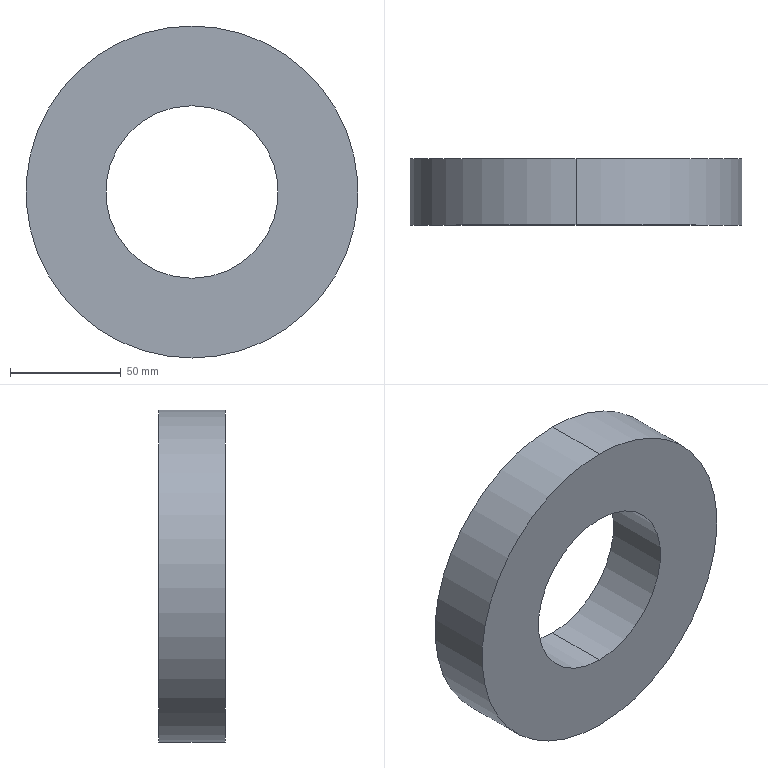Part | STEP file | Take-up roll | 1 solid | 6 faces | box 150 x 30 x 150 mm | volume 386793 mm3 | cylinder 4 | plane 2 | commonest cylinder face diameters 78 x2 150 x2
STEP:
#1=CARTESIAN_POINT('',(0.,0.,0.));
#2=DIRECTION('',(0.,0.,1.));
#3=DIRECTION('',(1.,0.,0.));
#4=AXIS2_PLACEMENT_3D('',#1,#2,#3);
#5=CARTESIAN_POINT('',(0.,15.,-39.));
#6=VERTEX_POINT('',#5);
#7=CARTESIAN_POINT('',(0.,-15.,-39.));
#8=VERTEX_POINT('',#7);
#9=CARTESIAN_POINT('',(0.,15.,-39.));
#10=DIRECTION('',(0.,-1.,0.));
#11=VECTOR('',#10,1.);
#12=LINE('',#9,#11);
#13=CARTESIAN_POINT('',(0.,15.,0.));
#14=DIRECTION('',(0.,-1.,0.));
#15=DIRECTION('',(0.,0.,-1.));
#16=AXIS2_PLACEMENT_3D('',#13,#14,#15);
#17=CYLINDRICAL_SURFACE('',#16,39.);
#18=CARTESIAN_POINT('',(6.283,0.));
#19=DIRECTION('',(0.,1.));
#20=VECTOR('',#19,1.);
#21=LINE('',#18,#20);
#22=(GEOMETRIC_REPRESENTATION_CONTEXT(2)PARAMETRIC_REPRESENTATION_CONTEXT()REPRESENTATION_CONTEXT('',''));
#23=DEFINITIONAL_REPRESENTATION('',(#21),#22);
#24=PCURVE('',#17,#23);
#25=CARTESIAN_POINT('',(0.,15.,0.));
#26=DIRECTION('',(0.,-1.,0.));
#27=DIRECTION('',(0.,0.,-1.));
#28=AXIS2_PLACEMENT_3D('',#25,#26,#27);
#29=CYLINDRICAL_SURFACE('',#28,39.);
#30=CARTESIAN_POINT('',(0.,0.));
#31=DIRECTION('',(0.,1.));
#32=VECTOR('',#31,1.);
#33=LINE('',#30,#32);
#34=(GEOMETRIC_REPRESENTATION_CONTEXT(2)PARAMETRIC_REPRESENTATION_CONTEXT()REPRESENTATION_CONTEXT('',''));
#35=DEFINITIONAL_REPRESENTATION('',(#33),#34);
#36=PCURVE('',#29,#35);
#37=SURFACE_CURVE('',#12,(#24,#36),.PCURVE_S1.);
#38=EDGE_CURVE('',#6,#8,#37,.T.);
#39=ORIENTED_EDGE('',*,*,#38,.T.);
#40=CARTESIAN_POINT('',(0.,-15.,39.));
#41=VERTEX_POINT('',#40);
#42=CARTESIAN_POINT('',(0.,-15.,0.));
#43=DIRECTION('',(0.,-1.,0.));
#44=DIRECTION('',(0.,0.,-1.));
#45=AXIS2_PLACEMENT_3D('',#42,#43,#44);
#46=CIRCLE('',#45,39.);
#47=CARTESIAN_POINT('',(0.,30.));
#48=DIRECTION('',(1.,0.));
#49=VECTOR('',#48,1.);
#50=LINE('',#47,#49);
#51=(GEOMETRIC_REPRESENTATION_CONTEXT(2)PARAMETRIC_REPRESENTATION_CONTEXT()REPRESENTATION_CONTEXT('',''));
#52=DEFINITIONAL_REPRESENTATION('',(#50),#51);
#53=PCURVE('',#17,#52);
#54=CARTESIAN_POINT('',(0.,-15.,0.));
#55=DIRECTION('',(0.,1.,0.));
#56=DIRECTION('',(0.,0.,1.));
#57=AXIS2_PLACEMENT_3D('',#54,#55,#56);
#58=PLANE('',#57);
#59=CARTESIAN_POINT('',(-39.,0.));
#60=CARTESIAN_POINT('',(-39.,67.55));
#61=CARTESIAN_POINT('',(19.5,33.775));
#62=CARTESIAN_POINT('',(78.,0.));
#63=CARTESIAN_POINT('',(19.5,-33.775));
#64=CARTESIAN_POINT('',(-39.,-67.55));
#65=CARTESIAN_POINT('',(-39.,0.));
#66=(BOUNDED_CURVE()B_SPLINE_CURVE(2,(#59,#60,#61,#62,#63,#64,#65),.UNSPECIFIED.,.T.,.F.)B_SPLINE_CURVE_WITH_KNOTS((1,2,2,2,2,1),(-2.094,0.,2.094,4.189,6.283,8.378),.UNSPECIFIED.)CURVE()GEOMETRIC_REPRESENTATION_ITEM()RATIONAL_B_SPLINE_CURVE((1.,0.5,1.,0.5,1.,0.5,1.))REPRESENTATION_ITEM(''));
#67=(GEOMETRIC_REPRESENTATION_CONTEXT(2)PARAMETRIC_REPRESENTATION_CONTEXT()REPRESENTATION_CONTEXT('',''));
#68=DEFINITIONAL_REPRESENTATION('',(#66),#67);
#69=PCURVE('',#58,#68);
#70=SURFACE_CURVE('',#46,(#53,#69),.PCURVE_S1.);
#71=EDGE_CURVE('',#41,#8,#70,.T.);
#72=ORIENTED_EDGE('',*,*,#71,.F.);
#73=CARTESIAN_POINT('',(0.,15.,39.));
#74=VERTEX_POINT('',#73);
#75=CARTESIAN_POINT('',(0.,15.,39.));
#76=DIRECTION('',(0.,-1.,0.));
#77=VECTOR('',#76,1.);
#78=LINE('',#75,#77);
#79=CARTESIAN_POINT('',(3.142,0.));
#80=DIRECTION('',(0.,1.));
#81=VECTOR('',#80,1.);
#82=LINE('',#79,#81);
#83=(GEOMETRIC_REPRESENTATION_CONTEXT(2)PARAMETRIC_REPRESENTATION_CONTEXT()REPRESENTATION_CONTEXT('',''));
#84=DEFINITIONAL_REPRESENTATION('',(#82),#83);
#85=PCURVE('',#17,#84);
#86=CARTESIAN_POINT('',(3.142,0.));
#87=DIRECTION('',(0.,1.));
#88=VECTOR('',#87,1.);
#89=LINE('',#86,#88);
#90=(GEOMETRIC_REPRESENTATION_CONTEXT(2)PARAMETRIC_REPRESENTATION_CONTEXT()REPRESENTATION_CONTEXT('',''));
#91=DEFINITIONAL_REPRESENTATION('',(#89),#90);
#92=PCURVE('',#29,#91);
#93=SURFACE_CURVE('',#78,(#85,#92),.PCURVE_S1.);
#94=EDGE_CURVE('',#74,#41,#93,.T.);
#95=ORIENTED_EDGE('',*,*,#94,.F.);
#96=CARTESIAN_POINT('',(0.,15.,0.));
#97=DIRECTION('',(0.,-1.,0.));
#98=DIRECTION('',(0.,0.,-1.));
#99=AXIS2_PLACEMENT_3D('',#96,#97,#98);
#100=CIRCLE('',#99,39.);
#101=CARTESIAN_POINT('',(0.,0.));
#102=DIRECTION('',(1.,0.));
#103=VECTOR('',#102,1.);
#104=LINE('',#101,#103);
#105=(GEOMETRIC_REPRESENTATION_CONTEXT(2)PARAMETRIC_REPRESENTATION_CONTEXT()REPRESENTATION_CONTEXT('',''));
#106=DEFINITIONAL_REPRESENTATION('',(#104),#105);
#107=PCURVE('',#17,#106);
#108=CARTESIAN_POINT('',(0.,15.,0.));
#109=DIRECTION('',(0.,1.,0.));
#110=DIRECTION('',(0.,0.,1.));
#111=AXIS2_PLACEMENT_3D('',#108,#109,#110);
#112=PLANE('',#111);
#113=CARTESIAN_POINT('',(-39.,0.));
#114=CARTESIAN_POINT('',(-39.,67.55));
#115=CARTESIAN_POINT('',(19.5,33.775));
#116=CARTESIAN_POINT('',(78.,0.));
#117=CARTESIAN_POINT('',(19.5,-33.775));
#118=CARTESIAN_POINT('',(-39.,-67.55));
#119=CARTESIAN_POINT('',(-39.,0.));
#120=(BOUNDED_CURVE()B_SPLINE_CURVE(2,(#113,#114,#115,#116,#117,#118,#119),.UNSPECIFIED.,.T.,.F.)B_SPLINE_CURVE_WITH_KNOTS((1,2,2,2,2,1),(-2.094,0.,2.094,4.189,6.283,8.378),.UNSPECIFIED.)CURVE()GEOMETRIC_REPRESENTATION_ITEM()RATIONAL_B_SPLINE_CURVE((1.,0.5,1.,0.5,1.,0.5,1.))REPRESENTATION_ITEM(''));
#121=(GEOMETRIC_REPRESENTATION_CONTEXT(2)PARAMETRIC_REPRESENTATION_CONTEXT()REPRESENTATION_CONTEXT('',''));
#122=DEFINITIONAL_REPRESENTATION('',(#120),#121);
#123=PCURVE('',#112,#122);
#124=SURFACE_CURVE('',#100,(#107,#123),.PCURVE_S1.);
#125=EDGE_CURVE('',#74,#6,#124,.T.);
#126=ORIENTED_EDGE('',*,*,#125,.T.);
#127=EDGE_LOOP('',(#39,#72,#95,#126));
#128=FACE_BOUND('',#127,.F.);
#129=ADVANCED_FACE('',(#128),#17,.F.);
#130=CARTESIAN_POINT('',(0.,15.,75.));
#131=VERTEX_POINT('',#130);
#132=CARTESIAN_POINT('',(0.,15.,-75.));
#133=VERTEX_POINT('',#132);
#134=CARTESIAN_POINT('',(0.,15.,0.));
#135=DIRECTION('',(0.,1.,0.));
#136=DIRECTION('',(0.,0.,1.));
#137=AXIS2_PLACEMENT_3D('',#134,#135,#136);
#138=CIRCLE('',#137,75.);
#139=CARTESIAN_POINT('',(0.,15.,0.));
#140=DIRECTION('',(0.,-1.,0.));
#141=DIRECTION('',(0.,0.,-1.));
#142=AXIS2_PLACEMENT_3D('',#139,#140,#141);
#143=CYLINDRICAL_SURFACE('',#142,75.);
#144=CARTESIAN_POINT('',(3.142,0.));
#145=DIRECTION('',(-1.,0.));
#146=VECTOR('',#145,1.);
#147=LINE('',#144,#146);
#148=(GEOMETRIC_REPRESENTATION_CONTEXT(2)PARAMETRIC_REPRESENTATION_CONTEXT()REPRESENTATION_CONTEXT('',''));
#149=DEFINITIONAL_REPRESENTATION('',(#147),#148);
#150=PCURVE('',#143,#149);
#151=CARTESIAN_POINT('',(0.,0.));
#152=DIRECTION('',(1.,0.));
#153=AXIS2_PLACEMENT_2D('',#151,#152);
#154=CIRCLE('',#153,75.);
#155=(GEOMETRIC_REPRESENTATION_CONTEXT(2)PARAMETRIC_REPRESENTATION_CONTEXT()REPRESENTATION_CONTEXT('',''));
#156=DEFINITIONAL_REPRESENTATION('',(#154),#155);
#157=PCURVE('',#112,#156);
#158=SURFACE_CURVE('',#138,(#150,#157),.PCURVE_S1.);
#159=EDGE_CURVE('',#131,#133,#158,.T.);
#160=ORIENTED_EDGE('',*,*,#159,.F.);
#161=CARTESIAN_POINT('',(0.,-15.,75.));
#162=VERTEX_POINT('',#161);
#163=CARTESIAN_POINT('',(0.,15.,75.));
#164=DIRECTION('',(0.,-1.,0.));
#165=VECTOR('',#164,1.);
#166=LINE('',#163,#165);
#167=CARTESIAN_POINT('',(3.142,0.));
#168=DIRECTION('',(0.,1.));
#169=VECTOR('',#168,1.);
#170=LINE('',#167,#169);
#171=(GEOMETRIC_REPRESENTATION_CONTEXT(2)PARAMETRIC_REPRESENTATION_CONTEXT()REPRESENTATION_CONTEXT('',''));
#172=DEFINITIONAL_REPRESENTATION('',(#170),#171);
#173=PCURVE('',#143,#172);
#174=CARTESIAN_POINT('',(0.,15.,0.));
#175=DIRECTION('',(0.,-1.,0.));
#176=DIRECTION('',(0.,0.,-1.));
#177=AXIS2_PLACEMENT_3D('',#174,#175,#176);
#178=CYLINDRICAL_SURFACE('',#177,75.);
#179=CARTESIAN_POINT('',(3.142,0.));
#180=DIRECTION('',(0.,1.));
#181=VECTOR('',#180,1.);
#182=LINE('',#179,#181);
#183=(GEOMETRIC_REPRESENTATION_CONTEXT(2)PARAMETRIC_REPRESENTATION_CONTEXT()REPRESENTATION_CONTEXT('',''));
#184=DEFINITIONAL_REPRESENTATION('',(#182),#183);
#185=PCURVE('',#178,#184);
#186=SURFACE_CURVE('',#166,(#173,#185),.PCURVE_S1.);
#187=EDGE_CURVE('',#131,#162,#186,.T.);
#188=ORIENTED_EDGE('',*,*,#187,.T.);
#189=CARTESIAN_POINT('',(0.,-15.,-75.));
#190=VERTEX_POINT('',#189);
#191=CARTESIAN_POINT('',(0.,-15.,0.));
#192=DIRECTION('',(0.,1.,0.));
#193=DIRECTION('',(0.,0.,1.));
#194=AXIS2_PLACEMENT_3D('',#191,#192,#193);
#195=CIRCLE('',#194,75.);
#196=CARTESIAN_POINT('',(3.142,30.));
#197=DIRECTION('',(-1.,0.));
#198=VECTOR('',#197,1.);
#199=LINE('',#196,#198);
#200=(GEOMETRIC_REPRESENTATION_CONTEXT(2)PARAMETRIC_REPRESENTATION_CONTEXT()REPRESENTATION_CONTEXT('',''));
#201=DEFINITIONAL_REPRESENTATION('',(#199),#200);
#202=PCURVE('',#143,#201);
#203=CARTESIAN_POINT('',(0.,0.));
#204=DIRECTION('',(1.,0.));
#205=AXIS2_PLACEMENT_2D('',#203,#204);
#206=CIRCLE('',#205,75.);
#207=(GEOMETRIC_REPRESENTATION_CONTEXT(2)PARAMETRIC_REPRESENTATION_CONTEXT()REPRESENTATION_CONTEXT('',''));
#208=DEFINITIONAL_REPRESENTATION('',(#206),#207);
#209=PCURVE('',#58,#208);
#210=SURFACE_CURVE('',#195,(#202,#209),.PCURVE_S1.);
#211=EDGE_CURVE('',#162,#190,#210,.T.);
#212=ORIENTED_EDGE('',*,*,#211,.T.);
#213=CARTESIAN_POINT('',(0.,15.,-75.));
#214=DIRECTION('',(0.,-1.,0.));
#215=VECTOR('',#214,1.);
#216=LINE('',#213,#215);
#217=CARTESIAN_POINT('',(0.,0.));
#218=DIRECTION('',(0.,1.));
#219=VECTOR('',#218,1.);
#220=LINE('',#217,#219);
#221=(GEOMETRIC_REPRESENTATION_CONTEXT(2)PARAMETRIC_REPRESENTATION_CONTEXT()REPRESENTATION_CONTEXT('',''));
#222=DEFINITIONAL_REPRESENTATION('',(#220),#221);
#223=PCURVE('',#143,#222);
#224=CARTESIAN_POINT('',(6.283,0.));
#225=DIRECTION('',(0.,1.));
#226=VECTOR('',#225,1.);
#227=LINE('',#224,#226);
#228=(GEOMETRIC_REPRESENTATION_CONTEXT(2)PARAMETRIC_REPRESENTATION_CONTEXT()REPRESENTATION_CONTEXT('',''));
#229=DEFINITIONAL_REPRESENTATION('',(#227),#228);
#230=PCURVE('',#178,#229);
#231=SURFACE_CURVE('',#216,(#223,#230),.PCURVE_S1.);
#232=EDGE_CURVE('',#133,#190,#231,.T.);
#233=ORIENTED_EDGE('',*,*,#232,.F.);
#234=EDGE_LOOP('',(#160,#188,#212,#233));
#235=FACE_BOUND('',#234,.T.);
#236=ADVANCED_FACE('',(#235),#143,.T.);
#237=ORIENTED_EDGE('',*,*,#187,.F.);
#238=CARTESIAN_POINT('',(0.,15.,0.));
#239=DIRECTION('',(0.,1.,0.));
#240=DIRECTION('',(0.,0.,1.));
#241=AXIS2_PLACEMENT_3D('',#238,#239,#240);
#242=CIRCLE('',#241,75.);
#243=CARTESIAN_POINT('',(9.425,0.));
#244=DIRECTION('',(-1.,0.));
#245=VECTOR('',#244,1.);
#246=LINE('',#243,#245);
#247=(GEOMETRIC_REPRESENTATION_CONTEXT(2)PARAMETRIC_REPRESENTATION_CONTEXT()REPRESENTATION_CONTEXT('',''));
#248=DEFINITIONAL_REPRESENTATION('',(#246),#247);
#249=PCURVE('',#178,#248);
#250=CARTESIAN_POINT('',(0.,0.));
#251=DIRECTION('',(1.,0.));
#252=AXIS2_PLACEMENT_2D('',#250,#251);
#253=CIRCLE('',#252,75.);
#254=(GEOMETRIC_REPRESENTATION_CONTEXT(2)PARAMETRIC_REPRESENTATION_CONTEXT()REPRESENTATION_CONTEXT('',''));
#255=DEFINITIONAL_REPRESENTATION('',(#253),#254);
#256=PCURVE('',#112,#255);
#257=SURFACE_CURVE('',#242,(#249,#256),.PCURVE_S1.);
#258=EDGE_CURVE('',#133,#131,#257,.T.);
#259=ORIENTED_EDGE('',*,*,#258,.F.);
#260=ORIENTED_EDGE('',*,*,#232,.T.);
#261=CARTESIAN_POINT('',(0.,-15.,0.));
#262=DIRECTION('',(0.,1.,0.));
#263=DIRECTION('',(0.,0.,1.));
#264=AXIS2_PLACEMENT_3D('',#261,#262,#263);
#265=CIRCLE('',#264,75.);
#266=CARTESIAN_POINT('',(9.425,30.));
#267=DIRECTION('',(-1.,0.));
#268=VECTOR('',#267,1.);
#269=LINE('',#266,#268);
#270=(GEOMETRIC_REPRESENTATION_CONTEXT(2)PARAMETRIC_REPRESENTATION_CONTEXT()REPRESENTATION_CONTEXT('',''));
#271=DEFINITIONAL_REPRESENTATION('',(#269),#270);
#272=PCURVE('',#178,#271);
#273=CARTESIAN_POINT('',(0.,0.));
#274=DIRECTION('',(1.,0.));
#275=AXIS2_PLACEMENT_2D('',#273,#274);
#276=CIRCLE('',#275,75.);
#277=(GEOMETRIC_REPRESENTATION_CONTEXT(2)PARAMETRIC_REPRESENTATION_CONTEXT()REPRESENTATION_CONTEXT('',''));
#278=DEFINITIONAL_REPRESENTATION('',(#276),#277);
#279=PCURVE('',#58,#278);
#280=SURFACE_CURVE('',#265,(#272,#279),.PCURVE_S1.);
#281=EDGE_CURVE('',#190,#162,#280,.T.);
#282=ORIENTED_EDGE('',*,*,#281,.T.);
#283=EDGE_LOOP('',(#237,#259,#260,#282));
#284=FACE_BOUND('',#283,.T.);
#285=ADVANCED_FACE('',(#284),#178,.T.);
#286=CARTESIAN_POINT('',(0.,15.,0.));
#287=DIRECTION('',(0.,-1.,0.));
#288=DIRECTION('',(0.,0.,-1.));
#289=AXIS2_PLACEMENT_3D('',#286,#287,#288);
#290=CIRCLE('',#289,39.);
#291=CARTESIAN_POINT('',(-39.,0.));
#292=CARTESIAN_POINT('',(-39.,67.55));
#293=CARTESIAN_POINT('',(19.5,33.775));
#294=CARTESIAN_POINT('',(78.,0.));
#295=CARTESIAN_POINT('',(19.5,-33.775));
#296=CARTESIAN_POINT('',(-39.,-67.55));
#297=CARTESIAN_POINT('',(-39.,0.));
#298=(BOUNDED_CURVE()B_SPLINE_CURVE(2,(#291,#292,#293,#294,#295,#296,#297),.UNSPECIFIED.,.T.,.F.)B_SPLINE_CURVE_WITH_KNOTS((1,2,2,2,2,1),(-2.094,0.,2.094,4.189,6.283,8.378),.UNSPECIFIED.)CURVE()GEOMETRIC_REPRESENTATION_ITEM()RATIONAL_B_SPLINE_CURVE((1.,0.5,1.,0.5,1.,0.5,1.))REPRESENTATION_ITEM(''));
#299=(GEOMETRIC_REPRESENTATION_CONTEXT(2)PARAMETRIC_REPRESENTATION_CONTEXT()REPRESENTATION_CONTEXT('',''));
#300=DEFINITIONAL_REPRESENTATION('',(#298),#299);
#301=PCURVE('',#112,#300);
#302=CARTESIAN_POINT('',(0.,0.));
#303=DIRECTION('',(1.,0.));
#304=VECTOR('',#303,1.);
#305=LINE('',#302,#304);
#306=(GEOMETRIC_REPRESENTATION_CONTEXT(2)PARAMETRIC_REPRESENTATION_CONTEXT()REPRESENTATION_CONTEXT('',''));
#307=DEFINITIONAL_REPRESENTATION('',(#305),#306);
#308=PCURVE('',#29,#307);
#309=SURFACE_CURVE('',#290,(#301,#308),.PCURVE_S1.);
#310=EDGE_CURVE('',#6,#74,#309,.T.);
#311=ORIENTED_EDGE('',*,*,#310,.T.);
#312=ORIENTED_EDGE('',*,*,#125,.T.);
#313=EDGE_LOOP('',(#311,#312));
#314=FACE_BOUND('',#313,.T.);
#315=ORIENTED_EDGE('',*,*,#258,.T.);
#316=ORIENTED_EDGE('',*,*,#159,.T.);
#317=EDGE_LOOP('',(#315,#316));
#318=FACE_BOUND('',#317,.T.);
#319=ADVANCED_FACE('',(#314,#318),#112,.T.);
#320=CARTESIAN_POINT('',(0.,-15.,0.));
#321=DIRECTION('',(0.,-1.,0.));
#322=DIRECTION('',(0.,0.,-1.));
#323=AXIS2_PLACEMENT_3D('',#320,#321,#322);
#324=CIRCLE('',#323,39.);
#325=CARTESIAN_POINT('',(-39.,0.));
#326=CARTESIAN_POINT('',(-39.,67.55));
#327=CARTESIAN_POINT('',(19.5,33.775));
#328=CARTESIAN_POINT('',(78.,0.));
#329=CARTESIAN_POINT('',(19.5,-33.775));
#330=CARTESIAN_POINT('',(-39.,-67.55));
#331=CARTESIAN_POINT('',(-39.,0.));
#332=(BOUNDED_CURVE()B_SPLINE_CURVE(2,(#325,#326,#327,#328,#329,#330,#331),.UNSPECIFIED.,.T.,.F.)B_SPLINE_CURVE_WITH_KNOTS((1,2,2,2,2,1),(-2.094,0.,2.094,4.189,6.283,8.378),.UNSPECIFIED.)CURVE()GEOMETRIC_REPRESENTATION_ITEM()RATIONAL_B_SPLINE_CURVE((1.,0.5,1.,0.5,1.,0.5,1.))REPRESENTATION_ITEM(''));
#333=(GEOMETRIC_REPRESENTATION_CONTEXT(2)PARAMETRIC_REPRESENTATION_CONTEXT()REPRESENTATION_CONTEXT('',''));
#334=DEFINITIONAL_REPRESENTATION('',(#332),#333);
#335=PCURVE('',#58,#334);
#336=CARTESIAN_POINT('',(0.,30.));
#337=DIRECTION('',(1.,0.));
#338=VECTOR('',#337,1.);
#339=LINE('',#336,#338);
#340=(GEOMETRIC_REPRESENTATION_CONTEXT(2)PARAMETRIC_REPRESENTATION_CONTEXT()REPRESENTATION_CONTEXT('',''));
#341=DEFINITIONAL_REPRESENTATION('',(#339),#340);
#342=PCURVE('',#29,#341);
#343=SURFACE_CURVE('',#324,(#335,#342),.PCURVE_S1.);
#344=EDGE_CURVE('',#8,#41,#343,.T.);
#345=ORIENTED_EDGE('',*,*,#344,.F.);
#346=ORIENTED_EDGE('',*,*,#71,.F.);
#347=EDGE_LOOP('',(#345,#346));
#348=FACE_BOUND('',#347,.T.);
#349=ORIENTED_EDGE('',*,*,#281,.F.);
#350=ORIENTED_EDGE('',*,*,#211,.F.);
#351=EDGE_LOOP('',(#349,#350));
#352=FACE_BOUND('',#351,.T.);
#353=ADVANCED_FACE('',(#348,#352),#58,.F.);
#354=ORIENTED_EDGE('',*,*,#344,.F.);
#355=ORIENTED_EDGE('',*,*,#38,.F.);
#356=ORIENTED_EDGE('',*,*,#310,.T.);
#357=ORIENTED_EDGE('',*,*,#94,.T.);
#358=EDGE_LOOP('',(#354,#355,#356,#357));
#359=FACE_BOUND('',#358,.F.);
#360=ADVANCED_FACE('',(#359),#29,.F.);
#361=CLOSED_SHELL('',(#129,#236,#285,#319,#353,#360));
#362=MANIFOLD_SOLID_BREP('',#361);
#363=(LENGTH_UNIT()NAMED_UNIT(*)SI_UNIT(.MILLI.,.METRE.));
#364=UNCERTAINTY_MEASURE_WITH_UNIT(LENGTH_MEASURE(0.0000001),#363,'','');
#365=(NAMED_UNIT(*)PLANE_ANGLE_UNIT()SI_UNIT($,.RADIAN.));
#366=(NAMED_UNIT(*)SI_UNIT($,.STERADIAN.)SOLID_ANGLE_UNIT());
#367=(GEOMETRIC_REPRESENTATION_CONTEXT(3)GLOBAL_UNCERTAINTY_ASSIGNED_CONTEXT((#364))GLOBAL_UNIT_ASSIGNED_CONTEXT((#363,#365,#366))REPRESENTATION_CONTEXT('',''));
#368=ADVANCED_BREP_SHAPE_REPRESENTATION('',(#4,#362),#367);